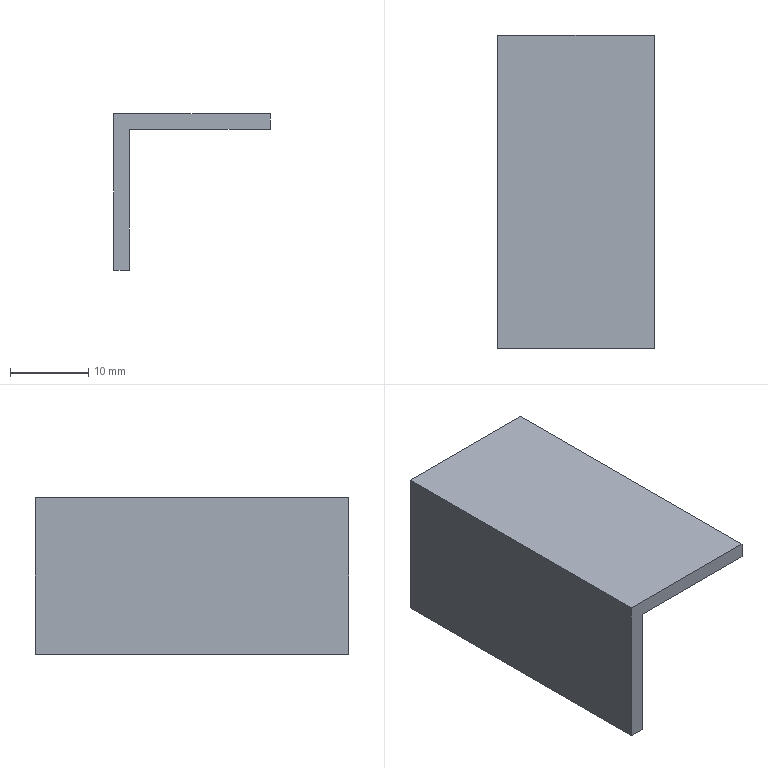Part | NX | 1 solid | 8 faces | box 20 x 40 x 20 mm | volume 3040 mm3 | plane 8
STEP:
#1=CARTESIAN_POINT('',(0.,0.,0.));
#2=VERTEX_POINT('',#1);
#3=CARTESIAN_POINT('',(20.,0.,0.));
#4=VERTEX_POINT('',#3);
#5=CARTESIAN_POINT('',(0.,0.,0.));
#6=DIRECTION('',(1.,0.,0.));
#7=VECTOR('',#6,1.);
#8=LINE('',#5,#7);
#9=EDGE_CURVE('',#2,#4,#8,.T.);
#10=ORIENTED_EDGE('',*,*,#9,.T.);
#11=CARTESIAN_POINT('',(20.,40.,0.));
#12=VERTEX_POINT('',#11);
#13=CARTESIAN_POINT('',(20.,40.,0.));
#14=DIRECTION('',(0.,-1.,0.));
#15=VECTOR('',#14,1.);
#16=LINE('',#13,#15);
#17=EDGE_CURVE('',#12,#4,#16,.T.);
#18=ORIENTED_EDGE('',*,*,#17,.F.);
#19=CARTESIAN_POINT('',(0.,40.,0.));
#20=VERTEX_POINT('',#19);
#21=CARTESIAN_POINT('',(0.,40.,0.));
#22=DIRECTION('',(1.,0.,0.));
#23=VECTOR('',#22,1.);
#24=LINE('',#21,#23);
#25=EDGE_CURVE('',#20,#12,#24,.T.);
#26=ORIENTED_EDGE('',*,*,#25,.F.);
#27=CARTESIAN_POINT('',(0.,40.,0.));
#28=DIRECTION('',(0.,-1.,0.));
#29=VECTOR('',#28,1.);
#30=LINE('',#27,#29);
#31=EDGE_CURVE('',#20,#2,#30,.T.);
#32=ORIENTED_EDGE('',*,*,#31,.T.);
#33=EDGE_LOOP('',(#10,#18,#26,#32));
#34=FACE_OUTER_BOUND('',#33,.T.);
#35=CARTESIAN_POINT('',(0.,40.,0.));
#36=DIRECTION('',(0.,0.,-1.));
#37=DIRECTION('',(-1.,0.,0.));
#38=AXIS2_PLACEMENT_3D('',#35,#36,#37);
#39=PLANE('',#38);
#40=ADVANCED_FACE('',(#34),#39,.F.);
#41=CARTESIAN_POINT('',(20.,0.,-2.));
#42=VERTEX_POINT('',#41);
#43=CARTESIAN_POINT('',(20.,0.,-2.));
#44=DIRECTION('',(0.,0.,-1.));
#45=VECTOR('',#44,1.);
#46=LINE('',#43,#45);
#47=EDGE_CURVE('',#4,#42,#46,.T.);
#48=ORIENTED_EDGE('',*,*,#47,.T.);
#49=CARTESIAN_POINT('',(20.,40.,-2.));
#50=VERTEX_POINT('',#49);
#51=CARTESIAN_POINT('',(20.,40.,-2.));
#52=DIRECTION('',(0.,-1.,0.));
#53=VECTOR('',#52,1.);
#54=LINE('',#51,#53);
#55=EDGE_CURVE('',#50,#42,#54,.T.);
#56=ORIENTED_EDGE('',*,*,#55,.F.);
#57=CARTESIAN_POINT('',(20.,40.,-2.));
#58=DIRECTION('',(0.,0.,-1.));
#59=VECTOR('',#58,1.);
#60=LINE('',#57,#59);
#61=EDGE_CURVE('',#12,#50,#60,.T.);
#62=ORIENTED_EDGE('',*,*,#61,.F.);
#63=ORIENTED_EDGE('',*,*,#17,.T.);
#64=EDGE_LOOP('',(#48,#56,#62,#63));
#65=FACE_OUTER_BOUND('',#64,.T.);
#66=CARTESIAN_POINT('',(20.,40.,-2.));
#67=DIRECTION('',(-1.,0.,0.));
#68=DIRECTION('',(0.,0.,1.));
#69=AXIS2_PLACEMENT_3D('',#66,#67,#68);
#70=PLANE('',#69);
#71=ADVANCED_FACE('',(#65),#70,.F.);
#72=CARTESIAN_POINT('',(2.,0.,-2.));
#73=VERTEX_POINT('',#72);
#74=CARTESIAN_POINT('',(2.,0.,-2.));
#75=DIRECTION('',(-1.,0.,0.));
#76=VECTOR('',#75,1.);
#77=LINE('',#74,#76);
#78=EDGE_CURVE('',#42,#73,#77,.T.);
#79=ORIENTED_EDGE('',*,*,#78,.T.);
#80=CARTESIAN_POINT('',(2.,40.,-2.));
#81=VERTEX_POINT('',#80);
#82=CARTESIAN_POINT('',(2.,40.,-2.));
#83=DIRECTION('',(0.,-1.,0.));
#84=VECTOR('',#83,1.);
#85=LINE('',#82,#84);
#86=EDGE_CURVE('',#81,#73,#85,.T.);
#87=ORIENTED_EDGE('',*,*,#86,.F.);
#88=CARTESIAN_POINT('',(2.,40.,-2.));
#89=DIRECTION('',(-1.,0.,0.));
#90=VECTOR('',#89,1.);
#91=LINE('',#88,#90);
#92=EDGE_CURVE('',#50,#81,#91,.T.);
#93=ORIENTED_EDGE('',*,*,#92,.F.);
#94=ORIENTED_EDGE('',*,*,#55,.T.);
#95=EDGE_LOOP('',(#79,#87,#93,#94));
#96=FACE_OUTER_BOUND('',#95,.T.);
#97=CARTESIAN_POINT('',(2.,40.,-2.));
#98=DIRECTION('',(0.,0.,1.));
#99=DIRECTION('',(1.,0.,0.));
#100=AXIS2_PLACEMENT_3D('',#97,#98,#99);
#101=PLANE('',#100);
#102=ADVANCED_FACE('',(#96),#101,.F.);
#103=CARTESIAN_POINT('',(2.,0.,-20.));
#104=VERTEX_POINT('',#103);
#105=CARTESIAN_POINT('',(2.,0.,-2.));
#106=DIRECTION('',(0.,0.,-1.));
#107=VECTOR('',#106,1.);
#108=LINE('',#105,#107);
#109=EDGE_CURVE('',#73,#104,#108,.T.);
#110=ORIENTED_EDGE('',*,*,#109,.T.);
#111=CARTESIAN_POINT('',(2.,40.,-20.));
#112=VERTEX_POINT('',#111);
#113=CARTESIAN_POINT('',(2.,40.,-20.));
#114=DIRECTION('',(0.,-1.,0.));
#115=VECTOR('',#114,1.);
#116=LINE('',#113,#115);
#117=EDGE_CURVE('',#112,#104,#116,.T.);
#118=ORIENTED_EDGE('',*,*,#117,.F.);
#119=CARTESIAN_POINT('',(2.,40.,-2.));
#120=DIRECTION('',(0.,0.,-1.));
#121=VECTOR('',#120,1.);
#122=LINE('',#119,#121);
#123=EDGE_CURVE('',#81,#112,#122,.T.);
#124=ORIENTED_EDGE('',*,*,#123,.F.);
#125=ORIENTED_EDGE('',*,*,#86,.T.);
#126=EDGE_LOOP('',(#110,#118,#124,#125));
#127=FACE_OUTER_BOUND('',#126,.T.);
#128=CARTESIAN_POINT('',(2.,40.,-2.));
#129=DIRECTION('',(-1.,0.,0.));
#130=DIRECTION('',(0.,0.,1.));
#131=AXIS2_PLACEMENT_3D('',#128,#129,#130);
#132=PLANE('',#131);
#133=ADVANCED_FACE('',(#127),#132,.F.);
#134=CARTESIAN_POINT('',(0.,0.,-20.));
#135=VERTEX_POINT('',#134);
#136=CARTESIAN_POINT('',(0.,0.,-20.));
#137=DIRECTION('',(-1.,0.,0.));
#138=VECTOR('',#137,1.);
#139=LINE('',#136,#138);
#140=EDGE_CURVE('',#104,#135,#139,.T.);
#141=ORIENTED_EDGE('',*,*,#140,.T.);
#142=CARTESIAN_POINT('',(0.,40.,-20.));
#143=VERTEX_POINT('',#142);
#144=CARTESIAN_POINT('',(0.,40.,-20.));
#145=DIRECTION('',(0.,-1.,0.));
#146=VECTOR('',#145,1.);
#147=LINE('',#144,#146);
#148=EDGE_CURVE('',#143,#135,#147,.T.);
#149=ORIENTED_EDGE('',*,*,#148,.F.);
#150=CARTESIAN_POINT('',(0.,40.,-20.));
#151=DIRECTION('',(-1.,0.,0.));
#152=VECTOR('',#151,1.);
#153=LINE('',#150,#152);
#154=EDGE_CURVE('',#112,#143,#153,.T.);
#155=ORIENTED_EDGE('',*,*,#154,.F.);
#156=ORIENTED_EDGE('',*,*,#117,.T.);
#157=EDGE_LOOP('',(#141,#149,#155,#156));
#158=FACE_OUTER_BOUND('',#157,.T.);
#159=CARTESIAN_POINT('',(0.,40.,-20.));
#160=DIRECTION('',(0.,0.,1.));
#161=DIRECTION('',(1.,0.,0.));
#162=AXIS2_PLACEMENT_3D('',#159,#160,#161);
#163=PLANE('',#162);
#164=ADVANCED_FACE('',(#158),#163,.F.);
#165=CARTESIAN_POINT('',(0.,0.,0.));
#166=DIRECTION('',(0.,0.,1.));
#167=VECTOR('',#166,1.);
#168=LINE('',#165,#167);
#169=EDGE_CURVE('',#135,#2,#168,.T.);
#170=ORIENTED_EDGE('',*,*,#169,.T.);
#171=ORIENTED_EDGE('',*,*,#31,.F.);
#172=CARTESIAN_POINT('',(0.,40.,0.));
#173=DIRECTION('',(0.,0.,1.));
#174=VECTOR('',#173,1.);
#175=LINE('',#172,#174);
#176=EDGE_CURVE('',#143,#20,#175,.T.);
#177=ORIENTED_EDGE('',*,*,#176,.F.);
#178=ORIENTED_EDGE('',*,*,#148,.T.);
#179=EDGE_LOOP('',(#170,#171,#177,#178));
#180=FACE_OUTER_BOUND('',#179,.T.);
#181=CARTESIAN_POINT('',(0.,40.,0.));
#182=DIRECTION('',(1.,0.,0.));
#183=DIRECTION('',(0.,0.,-1.));
#184=AXIS2_PLACEMENT_3D('',#181,#182,#183);
#185=PLANE('',#184);
#186=ADVANCED_FACE('',(#180),#185,.F.);
#187=ORIENTED_EDGE('',*,*,#25,.T.);
#188=ORIENTED_EDGE('',*,*,#61,.T.);
#189=ORIENTED_EDGE('',*,*,#92,.T.);
#190=ORIENTED_EDGE('',*,*,#123,.T.);
#191=ORIENTED_EDGE('',*,*,#154,.T.);
#192=ORIENTED_EDGE('',*,*,#176,.T.);
#193=EDGE_LOOP('',(#187,#188,#189,#190,#191,#192));
#194=FACE_OUTER_BOUND('',#193,.T.);
#195=CARTESIAN_POINT('',(20.,40.,0.));
#196=DIRECTION('',(0.,-1.,0.));
#197=DIRECTION('',(0.,0.,-1.));
#198=AXIS2_PLACEMENT_3D('',#195,#196,#197);
#199=PLANE('',#198);
#200=ADVANCED_FACE('',(#194),#199,.F.);
#201=ORIENTED_EDGE('',*,*,#9,.F.);
#202=ORIENTED_EDGE('',*,*,#169,.F.);
#203=ORIENTED_EDGE('',*,*,#140,.F.);
#204=ORIENTED_EDGE('',*,*,#109,.F.);
#205=ORIENTED_EDGE('',*,*,#78,.F.);
#206=ORIENTED_EDGE('',*,*,#47,.F.);
#207=EDGE_LOOP('',(#201,#202,#203,#204,#205,#206));
#208=FACE_OUTER_BOUND('',#207,.T.);
#209=CARTESIAN_POINT('',(20.,0.,0.));
#210=DIRECTION('',(0.,-1.,0.));
#211=DIRECTION('',(0.,0.,-1.));
#212=AXIS2_PLACEMENT_3D('',#209,#210,#211);
#213=PLANE('',#212);
#214=ADVANCED_FACE('',(#208),#213,.T.);
#215=CLOSED_SHELL('',(#40,#71,#102,#133,#164,#186,#200,#214));
#216=MANIFOLD_SOLID_BREP('',#215);
#217=(LENGTH_UNIT()NAMED_UNIT(*)SI_UNIT(.MILLI.,.METRE.));
#218=UNCERTAINTY_MEASURE_WITH_UNIT(LENGTH_MEASURE(0.00002),#217,'','');
#219=(NAMED_UNIT(*)PLANE_ANGLE_UNIT()SI_UNIT($,.RADIAN.));
#220=PLANE_ANGLE_MEASURE_WITH_UNIT(PLANE_ANGLE_MEASURE(0.01745),#219);
#221=DIMENSIONAL_EXPONENTS(0.,0.,0.,0.,0.,0.,0.);
#222=(CONVERSION_BASED_UNIT('DEGREE',#220)NAMED_UNIT(#221)PLANE_ANGLE_UNIT());
#223=(NAMED_UNIT(*)SI_UNIT($,.STERADIAN.)SOLID_ANGLE_UNIT());
#224=(GEOMETRIC_REPRESENTATION_CONTEXT(3)GLOBAL_UNCERTAINTY_ASSIGNED_CONTEXT((#218))GLOBAL_UNIT_ASSIGNED_CONTEXT((#217,#222,#223))REPRESENTATION_CONTEXT('',''));
#225=ADVANCED_BREP_SHAPE_REPRESENTATION('',(#216),#224);